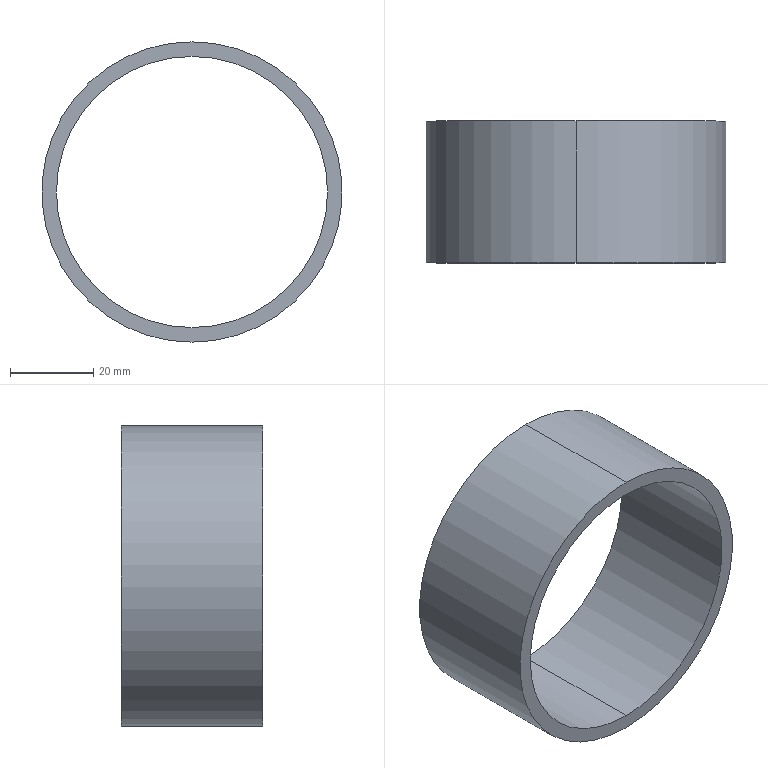Part | SolidWorks | features BaseBody 1 | 1 solid | 6 faces | box 72 x 34 x 72 mm | volume 25609 mm3 | cylinder 4 | plane 2 | commonest cylinder face diameters 65 x2 72 x2
STEP:
#1=CARTESIAN_POINT('',(0.,34.,-36.));
#2=VERTEX_POINT('',#1);
#3=CARTESIAN_POINT('',(0.,34.,36.));
#4=VERTEX_POINT('',#3);
#5=CARTESIAN_POINT('',(0.,34.,0.));
#6=DIRECTION('',(0.,-1.,0.));
#7=DIRECTION('',(0.,0.,-1.));
#8=AXIS2_PLACEMENT_3D('',#5,#6,#7);
#9=CIRCLE('',#8,36.);
#10=EDGE_CURVE('',#2,#4,#9,.T.);
#11=ORIENTED_EDGE('',*,*,#10,.T.);
#12=CARTESIAN_POINT('',(0.,0.,36.));
#13=VERTEX_POINT('',#12);
#14=CARTESIAN_POINT('',(0.,34.,36.));
#15=DIRECTION('',(0.,-1.,0.));
#16=VECTOR('',#15,1000.);
#17=LINE('',#14,#16);
#18=EDGE_CURVE('',#4,#13,#17,.T.);
#19=ORIENTED_EDGE('',*,*,#18,.T.);
#20=CARTESIAN_POINT('',(0.,0.,-36.));
#21=VERTEX_POINT('',#20);
#22=CARTESIAN_POINT('',(0.,0.,0.));
#23=DIRECTION('',(0.,1.,0.));
#24=DIRECTION('',(0.,0.,-1.));
#25=AXIS2_PLACEMENT_3D('',#22,#23,#24);
#26=CIRCLE('',#25,36.);
#27=EDGE_CURVE('',#13,#21,#26,.T.);
#28=ORIENTED_EDGE('',*,*,#27,.T.);
#29=CARTESIAN_POINT('',(0.,34.,-36.));
#30=DIRECTION('',(0.,-1.,0.));
#31=VECTOR('',#30,1000.);
#32=LINE('',#29,#31);
#33=EDGE_CURVE('',#2,#21,#32,.T.);
#34=ORIENTED_EDGE('',*,*,#33,.F.);
#35=EDGE_LOOP('',(#11,#19,#28,#34));
#36=FACE_OUTER_BOUND('',#35,.T.);
#37=CARTESIAN_POINT('',(0.,34.,0.));
#38=DIRECTION('',(0.,-1.,0.));
#39=DIRECTION('',(0.,0.,-1.));
#40=AXIS2_PLACEMENT_3D('',#37,#38,#39);
#41=CYLINDRICAL_SURFACE('',#40,36.);
#42=ADVANCED_FACE('',(#36),#41,.T.);
#43=CARTESIAN_POINT('',(0.,34.,32.5));
#44=VERTEX_POINT('',#43);
#45=CARTESIAN_POINT('',(0.,34.,-32.5));
#46=VERTEX_POINT('',#45);
#47=CARTESIAN_POINT('',(0.,34.,0.));
#48=DIRECTION('',(0.,-1.,0.));
#49=DIRECTION('',(0.,0.,-1.));
#50=AXIS2_PLACEMENT_3D('',#47,#48,#49);
#51=CIRCLE('',#50,32.5);
#52=EDGE_CURVE('',#44,#46,#51,.T.);
#53=ORIENTED_EDGE('',*,*,#52,.F.);
#54=CARTESIAN_POINT('',(0.,0.,32.5));
#55=VERTEX_POINT('',#54);
#56=CARTESIAN_POINT('',(0.,34.,32.5));
#57=DIRECTION('',(0.,-1.,0.));
#58=VECTOR('',#57,1000.);
#59=LINE('',#56,#58);
#60=EDGE_CURVE('',#44,#55,#59,.T.);
#61=ORIENTED_EDGE('',*,*,#60,.T.);
#62=CARTESIAN_POINT('',(0.,0.,-32.5));
#63=VERTEX_POINT('',#62);
#64=CARTESIAN_POINT('',(0.,0.,0.));
#65=DIRECTION('',(0.,-1.,0.));
#66=DIRECTION('',(0.,0.,-1.));
#67=AXIS2_PLACEMENT_3D('',#64,#65,#66);
#68=CIRCLE('',#67,32.5);
#69=EDGE_CURVE('',#55,#63,#68,.T.);
#70=ORIENTED_EDGE('',*,*,#69,.T.);
#71=CARTESIAN_POINT('',(0.,34.,-32.5));
#72=DIRECTION('',(0.,-1.,0.));
#73=VECTOR('',#72,1000.);
#74=LINE('',#71,#73);
#75=EDGE_CURVE('',#46,#63,#74,.T.);
#76=ORIENTED_EDGE('',*,*,#75,.F.);
#77=EDGE_LOOP('',(#53,#61,#70,#76));
#78=FACE_OUTER_BOUND('',#77,.T.);
#79=CARTESIAN_POINT('',(0.,34.,0.));
#80=DIRECTION('',(0.,-1.,0.));
#81=DIRECTION('',(0.,0.,-1.));
#82=AXIS2_PLACEMENT_3D('',#79,#80,#81);
#83=CYLINDRICAL_SURFACE('',#82,32.5);
#84=ADVANCED_FACE('',(#78),#83,.F.);
#85=ORIENTED_EDGE('',*,*,#18,.F.);
#86=CARTESIAN_POINT('',(0.,34.,0.));
#87=DIRECTION('',(0.,-1.,0.));
#88=DIRECTION('',(0.,0.,-1.));
#89=AXIS2_PLACEMENT_3D('',#86,#87,#88);
#90=CIRCLE('',#89,36.);
#91=EDGE_CURVE('',#4,#2,#90,.T.);
#92=ORIENTED_EDGE('',*,*,#91,.T.);
#93=ORIENTED_EDGE('',*,*,#33,.T.);
#94=CARTESIAN_POINT('',(0.,0.,0.));
#95=DIRECTION('',(0.,1.,0.));
#96=DIRECTION('',(0.,0.,-1.));
#97=AXIS2_PLACEMENT_3D('',#94,#95,#96);
#98=CIRCLE('',#97,36.);
#99=EDGE_CURVE('',#21,#13,#98,.T.);
#100=ORIENTED_EDGE('',*,*,#99,.T.);
#101=EDGE_LOOP('',(#85,#92,#93,#100));
#102=FACE_OUTER_BOUND('',#101,.T.);
#103=CARTESIAN_POINT('',(0.,34.,0.));
#104=DIRECTION('',(0.,-1.,0.));
#105=DIRECTION('',(0.,0.,-1.));
#106=AXIS2_PLACEMENT_3D('',#103,#104,#105);
#107=CYLINDRICAL_SURFACE('',#106,36.);
#108=ADVANCED_FACE('',(#102),#107,.T.);
#109=CARTESIAN_POINT('',(0.,0.,0.));
#110=DIRECTION('',(0.,-1.,0.));
#111=DIRECTION('',(0.,0.,-1.));
#112=AXIS2_PLACEMENT_3D('',#109,#110,#111);
#113=CIRCLE('',#112,32.5);
#114=EDGE_CURVE('',#63,#55,#113,.T.);
#115=ORIENTED_EDGE('',*,*,#114,.F.);
#116=ORIENTED_EDGE('',*,*,#69,.F.);
#117=EDGE_LOOP('',(#115,#116));
#118=FACE_BOUND('',#117,.T.);
#119=ORIENTED_EDGE('',*,*,#99,.F.);
#120=ORIENTED_EDGE('',*,*,#27,.F.);
#121=EDGE_LOOP('',(#119,#120));
#122=FACE_OUTER_BOUND('',#121,.T.);
#123=CARTESIAN_POINT('',(0.,0.,0.));
#124=DIRECTION('',(0.,1.,0.));
#125=DIRECTION('',(0.,0.,1.));
#126=AXIS2_PLACEMENT_3D('',#123,#124,#125);
#127=PLANE('',#126);
#128=ADVANCED_FACE('',(#118,#122),#127,.F.);
#129=CARTESIAN_POINT('',(0.,34.,0.));
#130=DIRECTION('',(0.,-1.,0.));
#131=DIRECTION('',(0.,0.,-1.));
#132=AXIS2_PLACEMENT_3D('',#129,#130,#131);
#133=CIRCLE('',#132,32.5);
#134=EDGE_CURVE('',#46,#44,#133,.T.);
#135=ORIENTED_EDGE('',*,*,#134,.T.);
#136=ORIENTED_EDGE('',*,*,#52,.T.);
#137=EDGE_LOOP('',(#135,#136));
#138=FACE_BOUND('',#137,.T.);
#139=ORIENTED_EDGE('',*,*,#10,.F.);
#140=ORIENTED_EDGE('',*,*,#91,.F.);
#141=EDGE_LOOP('',(#139,#140));
#142=FACE_OUTER_BOUND('',#141,.T.);
#143=CARTESIAN_POINT('',(0.,34.,0.));
#144=DIRECTION('',(0.,1.,0.));
#145=DIRECTION('',(0.,0.,1.));
#146=AXIS2_PLACEMENT_3D('',#143,#144,#145);
#147=PLANE('',#146);
#148=ADVANCED_FACE('',(#138,#142),#147,.T.);
#149=ORIENTED_EDGE('',*,*,#60,.F.);
#150=ORIENTED_EDGE('',*,*,#134,.F.);
#151=ORIENTED_EDGE('',*,*,#75,.T.);
#152=ORIENTED_EDGE('',*,*,#114,.T.);
#153=EDGE_LOOP('',(#149,#150,#151,#152));
#154=FACE_OUTER_BOUND('',#153,.T.);
#155=CARTESIAN_POINT('',(0.,34.,0.));
#156=DIRECTION('',(0.,-1.,0.));
#157=DIRECTION('',(0.,0.,-1.));
#158=AXIS2_PLACEMENT_3D('',#155,#156,#157);
#159=CYLINDRICAL_SURFACE('',#158,32.5);
#160=ADVANCED_FACE('',(#154),#159,.F.);
#161=CLOSED_SHELL('',(#42,#84,#108,#128,#148,#160));
#162=MANIFOLD_SOLID_BREP('',#161);
#163=CARTESIAN_POINT('',(0.,0.,0.));
#164=DIRECTION('',(0.,0.,1.));
#165=DIRECTION('',(1.,0.,0.));
#166=AXIS2_PLACEMENT_3D('',#163,#164,#165);
#167=(LENGTH_UNIT()NAMED_UNIT(*)SI_UNIT(.MILLI.,.METRE.));
#168=UNCERTAINTY_MEASURE_WITH_UNIT(LENGTH_MEASURE(0.00001),#167,'','');
#169=(NAMED_UNIT(*)PLANE_ANGLE_UNIT()SI_UNIT($,.RADIAN.));
#170=(NAMED_UNIT(*)SI_UNIT($,.STERADIAN.)SOLID_ANGLE_UNIT());
#171=(GEOMETRIC_REPRESENTATION_CONTEXT(3)GLOBAL_UNCERTAINTY_ASSIGNED_CONTEXT((#168))GLOBAL_UNIT_ASSIGNED_CONTEXT((#167,#169,#170))REPRESENTATION_CONTEXT('',''));
#172=ADVANCED_BREP_SHAPE_REPRESENTATION('',(#162,#166),#171);